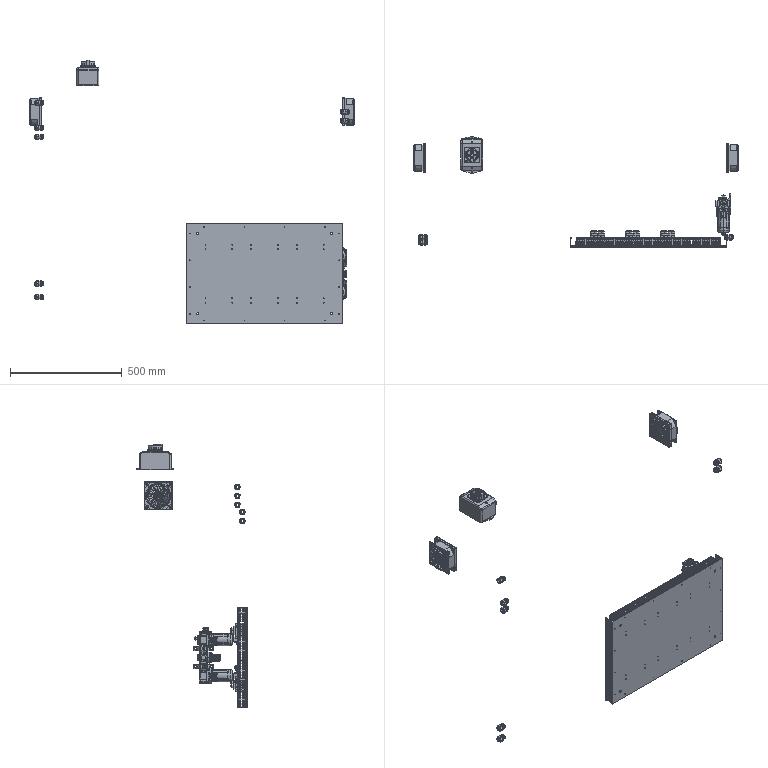Part | SolidWorks | features InContextFeatHolder 2, MirrorCompFeat 2 | 111 solids | 14156 faces | volume 6443563 mm3 | plane 6841 | cylinder 5508 | cone 992 | spline 596 | torus 202 | sphere 17 | commonest cylinder face diameters 5 x1843 2 x428 7.9 x192 4 x190 6.2 x144 8.57 x144